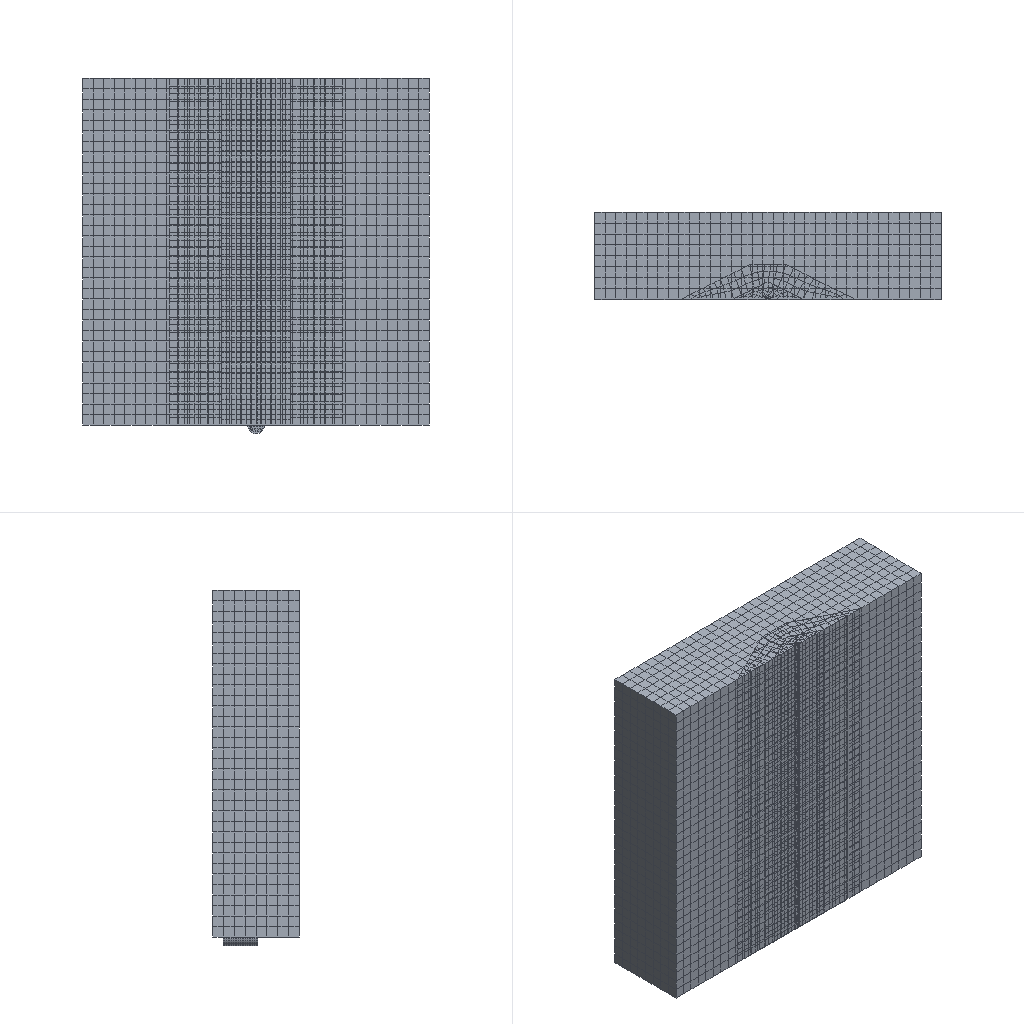Simulation study | abaqus
Set-up summary:
category,name,step,type,value,unit,region
solver,abaqus
solver,version,,,Abaqus/Explicit 2020
units,not stated in the deck,,not stated
analysis,deck,,transient,transient
load_step,Step-1,Step-1,transient,nlgeom=True
contact,interactions,,,general=0 pairs=1 ties=1
load_step,requested,,,1
mesh,nodes,,,27790
mesh,elements,,,21548
element_type,C3D8R,,solid,21548
load,load commands in deck,,count,1
bc,support commands in deck,,count,7
material,LV,,in results
material,MATERIAL-4,,in results
material,SOIL,,in results
material,SOIL-OUT,,in results
check,setup vs results,,match,"per instance, exact: element labels, types and connectivity; labels of the nodes the elements use; coordinates not compared"
Results summary:
result,step,Step-1,completed,increments=261 time=0.01/0.01
result,analysis,,,transient
result,last_loadstep,,,1
result,analysis steps,,count,1
result,primary field,,,U
result,reaction total,,FX,-5508391.001,model units
result,reaction total,,FY,-64315176.491,model units
result,reaction total,,FZ,44068964.212,model units